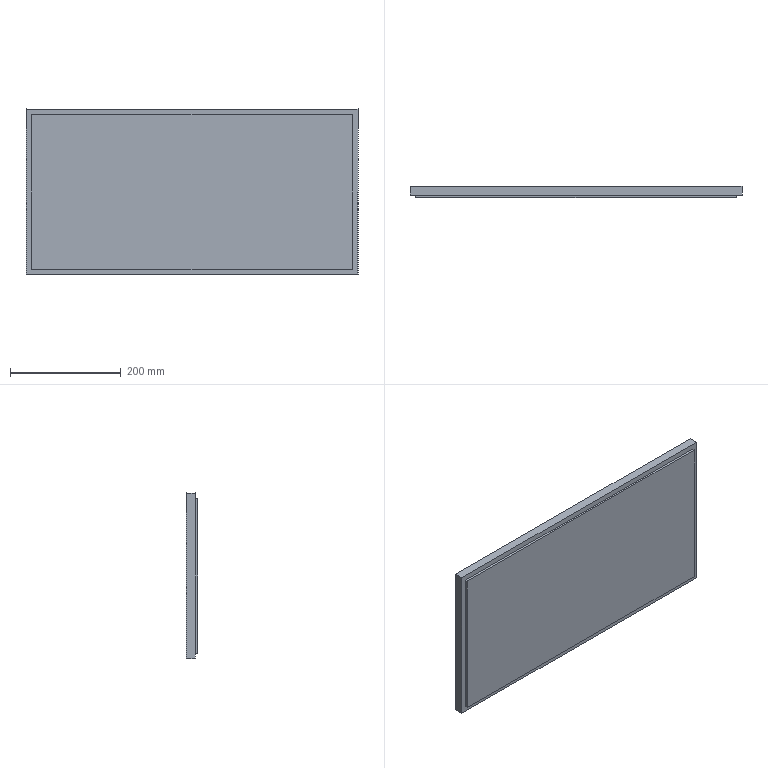Part | SolidWorks | features Extrusion 1, ICE 1 | 1 solid | 11 faces | box 600 x 20 x 300 mm | volume 3529600 mm3 | plane 11
STEP:
#1=CARTESIAN_POINT('',(300.,4.,-150.));
#2=VERTEX_POINT('',#1);
#3=CARTESIAN_POINT('',(300.,4.,150.));
#4=VERTEX_POINT('',#3);
#5=CARTESIAN_POINT('',(300.,4.,-150.));
#6=DIRECTION('',(0.,0.,1.));
#7=VECTOR('',#6,1000.);
#8=LINE('',#5,#7);
#9=EDGE_CURVE('',#2,#4,#8,.T.);
#10=ORIENTED_EDGE('',*,*,#9,.F.);
#11=CARTESIAN_POINT('',(300.,20.,-150.));
#12=VERTEX_POINT('',#11);
#13=CARTESIAN_POINT('',(300.,20.,-150.));
#14=DIRECTION('',(0.,-1.,0.));
#15=VECTOR('',#14,1000.);
#16=LINE('',#13,#15);
#17=EDGE_CURVE('',#12,#2,#16,.T.);
#18=ORIENTED_EDGE('',*,*,#17,.F.);
#19=CARTESIAN_POINT('',(300.,20.,150.));
#20=VERTEX_POINT('',#19);
#21=CARTESIAN_POINT('',(300.,20.,-150.));
#22=DIRECTION('',(0.,0.,-1.));
#23=VECTOR('',#22,1000.);
#24=LINE('',#21,#23);
#25=EDGE_CURVE('',#20,#12,#24,.T.);
#26=ORIENTED_EDGE('',*,*,#25,.F.);
#27=CARTESIAN_POINT('',(300.,20.,150.));
#28=DIRECTION('',(0.,-1.,0.));
#29=VECTOR('',#28,1000.);
#30=LINE('',#27,#29);
#31=EDGE_CURVE('',#20,#4,#30,.T.);
#32=ORIENTED_EDGE('',*,*,#31,.T.);
#33=EDGE_LOOP('',(#10,#18,#26,#32));
#34=FACE_OUTER_BOUND('',#33,.T.);
#35=CARTESIAN_POINT('',(300.,20.,-150.));
#36=DIRECTION('',(-1.,0.,0.));
#37=DIRECTION('',(0.,0.,1.));
#38=AXIS2_PLACEMENT_3D('',#35,#36,#37);
#39=PLANE('',#38);
#40=ADVANCED_FACE('',(#34),#39,.F.);
#41=CARTESIAN_POINT('',(-300.,4.,-150.));
#42=VERTEX_POINT('',#41);
#43=CARTESIAN_POINT('',(-300.,4.,-150.));
#44=DIRECTION('',(1.,0.,0.));
#45=VECTOR('',#44,1000.);
#46=LINE('',#43,#45);
#47=EDGE_CURVE('',#42,#2,#46,.T.);
#48=ORIENTED_EDGE('',*,*,#47,.F.);
#49=CARTESIAN_POINT('',(-300.,20.,-150.));
#50=VERTEX_POINT('',#49);
#51=CARTESIAN_POINT('',(-300.,20.,-150.));
#52=DIRECTION('',(0.,-1.,0.));
#53=VECTOR('',#52,1000.);
#54=LINE('',#51,#53);
#55=EDGE_CURVE('',#50,#42,#54,.T.);
#56=ORIENTED_EDGE('',*,*,#55,.F.);
#57=CARTESIAN_POINT('',(-300.,20.,-150.));
#58=DIRECTION('',(-1.,0.,0.));
#59=VECTOR('',#58,1000.);
#60=LINE('',#57,#59);
#61=EDGE_CURVE('',#12,#50,#60,.T.);
#62=ORIENTED_EDGE('',*,*,#61,.F.);
#63=ORIENTED_EDGE('',*,*,#17,.T.);
#64=EDGE_LOOP('',(#48,#56,#62,#63));
#65=FACE_OUTER_BOUND('',#64,.T.);
#66=CARTESIAN_POINT('',(-300.,20.,-150.));
#67=DIRECTION('',(0.,0.,1.));
#68=DIRECTION('',(1.,0.,0.));
#69=AXIS2_PLACEMENT_3D('',#66,#67,#68);
#70=PLANE('',#69);
#71=ADVANCED_FACE('',(#65),#70,.F.);
#72=CARTESIAN_POINT('',(-300.,4.,150.));
#73=VERTEX_POINT('',#72);
#74=CARTESIAN_POINT('',(-300.,4.,-150.));
#75=DIRECTION('',(0.,0.,-1.));
#76=VECTOR('',#75,1000.);
#77=LINE('',#74,#76);
#78=EDGE_CURVE('',#73,#42,#77,.T.);
#79=ORIENTED_EDGE('',*,*,#78,.F.);
#80=CARTESIAN_POINT('',(-300.,20.,150.));
#81=VERTEX_POINT('',#80);
#82=CARTESIAN_POINT('',(-300.,20.,150.));
#83=DIRECTION('',(0.,-1.,0.));
#84=VECTOR('',#83,1000.);
#85=LINE('',#82,#84);
#86=EDGE_CURVE('',#81,#73,#85,.T.);
#87=ORIENTED_EDGE('',*,*,#86,.F.);
#88=CARTESIAN_POINT('',(-300.,20.,-150.));
#89=DIRECTION('',(0.,0.,1.));
#90=VECTOR('',#89,1000.);
#91=LINE('',#88,#90);
#92=EDGE_CURVE('',#50,#81,#91,.T.);
#93=ORIENTED_EDGE('',*,*,#92,.F.);
#94=ORIENTED_EDGE('',*,*,#55,.T.);
#95=EDGE_LOOP('',(#79,#87,#93,#94));
#96=FACE_OUTER_BOUND('',#95,.T.);
#97=CARTESIAN_POINT('',(-300.,20.,-150.));
#98=DIRECTION('',(1.,0.,0.));
#99=DIRECTION('',(0.,0.,-1.));
#100=AXIS2_PLACEMENT_3D('',#97,#98,#99);
#101=PLANE('',#100);
#102=ADVANCED_FACE('',(#96),#101,.F.);
#103=CARTESIAN_POINT('',(-300.,4.,150.));
#104=DIRECTION('',(-1.,0.,0.));
#105=VECTOR('',#104,1000.);
#106=LINE('',#103,#105);
#107=EDGE_CURVE('',#4,#73,#106,.T.);
#108=ORIENTED_EDGE('',*,*,#107,.F.);
#109=ORIENTED_EDGE('',*,*,#31,.F.);
#110=CARTESIAN_POINT('',(-300.,20.,150.));
#111=DIRECTION('',(1.,0.,0.));
#112=VECTOR('',#111,1000.);
#113=LINE('',#110,#112);
#114=EDGE_CURVE('',#81,#20,#113,.T.);
#115=ORIENTED_EDGE('',*,*,#114,.F.);
#116=ORIENTED_EDGE('',*,*,#86,.T.);
#117=EDGE_LOOP('',(#108,#109,#115,#116));
#118=FACE_OUTER_BOUND('',#117,.T.);
#119=CARTESIAN_POINT('',(-300.,20.,150.));
#120=DIRECTION('',(0.,0.,-1.));
#121=DIRECTION('',(-1.,0.,0.));
#122=AXIS2_PLACEMENT_3D('',#119,#120,#121);
#123=PLANE('',#122);
#124=ADVANCED_FACE('',(#118),#123,.F.);
#125=ORIENTED_EDGE('',*,*,#25,.T.);
#126=ORIENTED_EDGE('',*,*,#61,.T.);
#127=ORIENTED_EDGE('',*,*,#92,.T.);
#128=ORIENTED_EDGE('',*,*,#114,.T.);
#129=EDGE_LOOP('',(#125,#126,#127,#128));
#130=FACE_OUTER_BOUND('',#129,.T.);
#131=CARTESIAN_POINT('',(0.,20.,0.));
#132=DIRECTION('',(0.,1.,0.));
#133=DIRECTION('',(0.,0.,1.));
#134=AXIS2_PLACEMENT_3D('',#131,#132,#133);
#135=PLANE('',#134);
#136=ADVANCED_FACE('',(#130),#135,.T.);
#137=CARTESIAN_POINT('',(-290.,4.,-140.));
#138=VERTEX_POINT('',#137);
#139=CARTESIAN_POINT('',(290.,4.,-140.));
#140=VERTEX_POINT('',#139);
#141=CARTESIAN_POINT('',(-290.,4.,-140.));
#142=DIRECTION('',(1.,0.,0.));
#143=VECTOR('',#142,1000.);
#144=LINE('',#141,#143);
#145=EDGE_CURVE('',#138,#140,#144,.T.);
#146=ORIENTED_EDGE('',*,*,#145,.F.);
#147=CARTESIAN_POINT('',(-290.,4.,140.));
#148=VERTEX_POINT('',#147);
#149=CARTESIAN_POINT('',(-290.,4.,140.));
#150=DIRECTION('',(0.,0.,-1.));
#151=VECTOR('',#150,1000.);
#152=LINE('',#149,#151);
#153=EDGE_CURVE('',#148,#138,#152,.T.);
#154=ORIENTED_EDGE('',*,*,#153,.F.);
#155=CARTESIAN_POINT('',(290.,4.,140.));
#156=VERTEX_POINT('',#155);
#157=CARTESIAN_POINT('',(-290.,4.,140.));
#158=DIRECTION('',(-1.,0.,0.));
#159=VECTOR('',#158,1000.);
#160=LINE('',#157,#159);
#161=EDGE_CURVE('',#156,#148,#160,.T.);
#162=ORIENTED_EDGE('',*,*,#161,.F.);
#163=CARTESIAN_POINT('',(290.,4.,140.));
#164=DIRECTION('',(0.,0.,1.));
#165=VECTOR('',#164,1000.);
#166=LINE('',#163,#165);
#167=EDGE_CURVE('',#140,#156,#166,.T.);
#168=ORIENTED_EDGE('',*,*,#167,.F.);
#169=EDGE_LOOP('',(#146,#154,#162,#168));
#170=FACE_BOUND('',#169,.T.);
#171=ORIENTED_EDGE('',*,*,#9,.T.);
#172=ORIENTED_EDGE('',*,*,#107,.T.);
#173=ORIENTED_EDGE('',*,*,#78,.T.);
#174=ORIENTED_EDGE('',*,*,#47,.T.);
#175=EDGE_LOOP('',(#171,#172,#173,#174));
#176=FACE_OUTER_BOUND('',#175,.T.);
#177=CARTESIAN_POINT('',(0.,4.,0.));
#178=DIRECTION('',(0.,-1.,0.));
#179=DIRECTION('',(0.,0.,-1.));
#180=AXIS2_PLACEMENT_3D('',#177,#178,#179);
#181=PLANE('',#180);
#182=ADVANCED_FACE('',(#170,#176),#181,.T.);
#183=CARTESIAN_POINT('',(290.,0.,-140.));
#184=VERTEX_POINT('',#183);
#185=CARTESIAN_POINT('',(290.,0.,140.));
#186=VERTEX_POINT('',#185);
#187=CARTESIAN_POINT('',(290.,0.,140.));
#188=DIRECTION('',(0.,0.,1.));
#189=VECTOR('',#188,1000.);
#190=LINE('',#187,#189);
#191=EDGE_CURVE('',#184,#186,#190,.T.);
#192=ORIENTED_EDGE('',*,*,#191,.F.);
#193=CARTESIAN_POINT('',(290.,4.,-140.));
#194=DIRECTION('',(0.,-1.,0.));
#195=VECTOR('',#194,1000.);
#196=LINE('',#193,#195);
#197=EDGE_CURVE('',#140,#184,#196,.T.);
#198=ORIENTED_EDGE('',*,*,#197,.F.);
#199=ORIENTED_EDGE('',*,*,#167,.T.);
#200=CARTESIAN_POINT('',(290.,4.,140.));
#201=DIRECTION('',(0.,-1.,0.));
#202=VECTOR('',#201,1000.);
#203=LINE('',#200,#202);
#204=EDGE_CURVE('',#156,#186,#203,.T.);
#205=ORIENTED_EDGE('',*,*,#204,.T.);
#206=EDGE_LOOP('',(#192,#198,#199,#205));
#207=FACE_OUTER_BOUND('',#206,.T.);
#208=CARTESIAN_POINT('',(290.,4.,140.));
#209=DIRECTION('',(1.,0.,0.));
#210=DIRECTION('',(0.,0.,-1.));
#211=AXIS2_PLACEMENT_3D('',#208,#209,#210);
#212=PLANE('',#211);
#213=ADVANCED_FACE('',(#207),#212,.T.);
#214=CARTESIAN_POINT('',(-290.,0.,-140.));
#215=VERTEX_POINT('',#214);
#216=CARTESIAN_POINT('',(-290.,0.,-140.));
#217=DIRECTION('',(1.,0.,0.));
#218=VECTOR('',#217,1000.);
#219=LINE('',#216,#218);
#220=EDGE_CURVE('',#215,#184,#219,.T.);
#221=ORIENTED_EDGE('',*,*,#220,.F.);
#222=CARTESIAN_POINT('',(-290.,4.,-140.));
#223=DIRECTION('',(0.,-1.,0.));
#224=VECTOR('',#223,1000.);
#225=LINE('',#222,#224);
#226=EDGE_CURVE('',#138,#215,#225,.T.);
#227=ORIENTED_EDGE('',*,*,#226,.F.);
#228=ORIENTED_EDGE('',*,*,#145,.T.);
#229=ORIENTED_EDGE('',*,*,#197,.T.);
#230=EDGE_LOOP('',(#221,#227,#228,#229));
#231=FACE_OUTER_BOUND('',#230,.T.);
#232=CARTESIAN_POINT('',(-290.,4.,-140.));
#233=DIRECTION('',(0.,0.,-1.));
#234=DIRECTION('',(-1.,0.,0.));
#235=AXIS2_PLACEMENT_3D('',#232,#233,#234);
#236=PLANE('',#235);
#237=ADVANCED_FACE('',(#231),#236,.T.);
#238=CARTESIAN_POINT('',(-290.,0.,140.));
#239=VERTEX_POINT('',#238);
#240=CARTESIAN_POINT('',(-290.,0.,140.));
#241=DIRECTION('',(0.,0.,-1.));
#242=VECTOR('',#241,1000.);
#243=LINE('',#240,#242);
#244=EDGE_CURVE('',#239,#215,#243,.T.);
#245=ORIENTED_EDGE('',*,*,#244,.F.);
#246=CARTESIAN_POINT('',(-290.,4.,140.));
#247=DIRECTION('',(0.,-1.,0.));
#248=VECTOR('',#247,1000.);
#249=LINE('',#246,#248);
#250=EDGE_CURVE('',#148,#239,#249,.T.);
#251=ORIENTED_EDGE('',*,*,#250,.F.);
#252=ORIENTED_EDGE('',*,*,#153,.T.);
#253=ORIENTED_EDGE('',*,*,#226,.T.);
#254=EDGE_LOOP('',(#245,#251,#252,#253));
#255=FACE_OUTER_BOUND('',#254,.T.);
#256=CARTESIAN_POINT('',(-290.,4.,140.));
#257=DIRECTION('',(-1.,0.,0.));
#258=DIRECTION('',(0.,0.,1.));
#259=AXIS2_PLACEMENT_3D('',#256,#257,#258);
#260=PLANE('',#259);
#261=ADVANCED_FACE('',(#255),#260,.T.);
#262=CARTESIAN_POINT('',(-290.,0.,140.));
#263=DIRECTION('',(-1.,0.,0.));
#264=VECTOR('',#263,1000.);
#265=LINE('',#262,#264);
#266=EDGE_CURVE('',#186,#239,#265,.T.);
#267=ORIENTED_EDGE('',*,*,#266,.F.);
#268=ORIENTED_EDGE('',*,*,#204,.F.);
#269=ORIENTED_EDGE('',*,*,#161,.T.);
#270=ORIENTED_EDGE('',*,*,#250,.T.);
#271=EDGE_LOOP('',(#267,#268,#269,#270));
#272=FACE_OUTER_BOUND('',#271,.T.);
#273=CARTESIAN_POINT('',(-290.,4.,140.));
#274=DIRECTION('',(0.,0.,1.));
#275=DIRECTION('',(1.,0.,0.));
#276=AXIS2_PLACEMENT_3D('',#273,#274,#275);
#277=PLANE('',#276);
#278=ADVANCED_FACE('',(#272),#277,.T.);
#279=ORIENTED_EDGE('',*,*,#191,.T.);
#280=ORIENTED_EDGE('',*,*,#266,.T.);
#281=ORIENTED_EDGE('',*,*,#244,.T.);
#282=ORIENTED_EDGE('',*,*,#220,.T.);
#283=EDGE_LOOP('',(#279,#280,#281,#282));
#284=FACE_OUTER_BOUND('',#283,.T.);
#285=CARTESIAN_POINT('',(0.,0.,0.));
#286=DIRECTION('',(0.,1.,0.));
#287=DIRECTION('',(0.,0.,1.));
#288=AXIS2_PLACEMENT_3D('',#285,#286,#287);
#289=PLANE('',#288);
#290=ADVANCED_FACE('',(#284),#289,.F.);
#291=CLOSED_SHELL('',(#40,#71,#102,#124,#136,#182,#213,#237,#261,#278,#290));
#292=MANIFOLD_SOLID_BREP('',#291);
#293=CARTESIAN_POINT('',(0.,0.,0.));
#294=DIRECTION('',(0.,0.,1.));
#295=DIRECTION('',(1.,0.,0.));
#296=AXIS2_PLACEMENT_3D('',#293,#294,#295);
#297=(LENGTH_UNIT()NAMED_UNIT(*)SI_UNIT(.MILLI.,.METRE.));
#298=UNCERTAINTY_MEASURE_WITH_UNIT(LENGTH_MEASURE(0.00001),#297,'','');
#299=(NAMED_UNIT(*)PLANE_ANGLE_UNIT()SI_UNIT($,.RADIAN.));
#300=(NAMED_UNIT(*)SI_UNIT($,.STERADIAN.)SOLID_ANGLE_UNIT());
#301=(GEOMETRIC_REPRESENTATION_CONTEXT(3)GLOBAL_UNCERTAINTY_ASSIGNED_CONTEXT((#298))GLOBAL_UNIT_ASSIGNED_CONTEXT((#297,#299,#300))REPRESENTATION_CONTEXT('',''));
#302=ADVANCED_BREP_SHAPE_REPRESENTATION('',(#292,#296),#301);